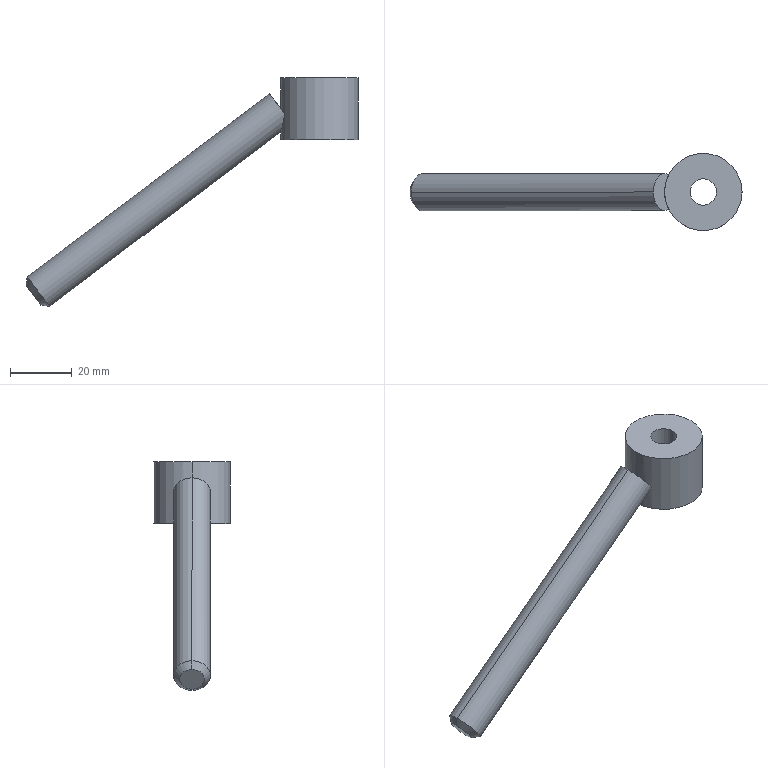Part | SolidWorks | features Chamfer 1, Extrusion 1, HoleWzd 1, Revolution 1 | 1 solid | 12 faces | box 107.206 x 25 x 73.855 mm | volume 19838 mm3 | cylinder 6 | plane 4 | cone 2 | commonest cylinder face diameters 8.5 x2 12 x2 25 x2
STEP:
#1=CARTESIAN_POINT('',(-94.706,0.,-57.081));
#2=VERTEX_POINT('',#1);
#3=CARTESIAN_POINT('',(-89.884,0.,-63.464));
#4=VERTEX_POINT('',#3);
#5=CARTESIAN_POINT('',(-92.295,0.,-60.273));
#6=DIRECTION('',(-0.7979,0.,-0.6027));
#7=DIRECTION('',(-0.6027,0.,0.7979));
#8=AXIS2_PLACEMENT_3D('',#5,#6,#7);
#9=CIRCLE('',#8,4.);
#10=EDGE_CURVE('',#2,#4,#9,.T.);
#11=ORIENTED_EDGE('',*,*,#10,.F.);
#12=CARTESIAN_POINT('',(-94.315,0.,-54.28));
#13=VERTEX_POINT('',#12);
#14=CARTESIAN_POINT('',(-94.315,0.,-54.28));
#15=DIRECTION('',(0.138,0.,0.9904));
#16=VECTOR('',#15,1000.);
#17=LINE('',#14,#16);
#18=EDGE_CURVE('',#2,#13,#17,.T.);
#19=ORIENTED_EDGE('',*,*,#18,.T.);
#20=CARTESIAN_POINT('',(-87.082,0.,-63.855));
#21=VERTEX_POINT('',#20);
#22=CARTESIAN_POINT('',(-90.699,0.,-59.067));
#23=DIRECTION('',(0.7979,0.,0.6027));
#24=DIRECTION('',(-0.6027,0.,0.7979));
#25=AXIS2_PLACEMENT_3D('',#22,#23,#24);
#26=CIRCLE('',#25,6.);
#27=EDGE_CURVE('',#21,#13,#26,.T.);
#28=ORIENTED_EDGE('',*,*,#27,.F.);
#29=CARTESIAN_POINT('',(-87.082,0.,-63.855));
#30=DIRECTION('',(0.9904,0.,-0.138));
#31=VECTOR('',#30,1000.);
#32=LINE('',#29,#31);
#33=EDGE_CURVE('',#4,#21,#32,.T.);
#34=ORIENTED_EDGE('',*,*,#33,.F.);
#35=EDGE_LOOP('',(#11,#19,#28,#34));
#36=FACE_OUTER_BOUND('',#35,.T.);
#37=CARTESIAN_POINT('',(-90.699,0.,-59.067));
#38=DIRECTION('',(0.7979,0.,0.6027));
#39=DIRECTION('',(0.6027,0.,-0.7979));
#40=AXIS2_PLACEMENT_3D('',#37,#38,#39);
#41=CONICAL_SURFACE('',#40,6.,0.7854);
#42=ADVANCED_FACE('',(#36),#41,.T.);
#43=ORIENTED_EDGE('',*,*,#27,.T.);
#44=CARTESIAN_POINT('',(-16.116,0.,4.788));
#45=VERTEX_POINT('',#44);
#46=CARTESIAN_POINT('',(-16.116,0.,4.788));
#47=DIRECTION('',(0.7979,0.,0.6027));
#48=VECTOR('',#47,1000.);
#49=LINE('',#46,#48);
#50=EDGE_CURVE('',#13,#45,#49,.T.);
#51=ORIENTED_EDGE('',*,*,#50,.T.);
#52=CARTESIAN_POINT('',(-11.182,5.587,-1.745));
#53=VERTEX_POINT('',#52);
#54=CARTESIAN_POINT('',(-12.5,0.,0.));
#55=DIRECTION('',(0.7979,0.,0.6027));
#56=DIRECTION('',(0.6027,0.,-0.7979));
#57=AXIS2_PLACEMENT_3D('',#54,#55,#56);
#58=CIRCLE('',#57,6.);
#59=EDGE_CURVE('',#53,#45,#58,.T.);
#60=ORIENTED_EDGE('',*,*,#59,.F.);
#61=CARTESIAN_POINT('',(-12.5,0.,-7.519));
#62=VERTEX_POINT('',#61);
#63=CARTESIAN_POINT('',(-12.5,0.,-7.519));
#64=CARTESIAN_POINT('',(-12.5,0.1816,-7.519));
#65=CARTESIAN_POINT('',(-12.496,0.362,-7.506));
#66=CARTESIAN_POINT('',(-12.481,0.7202,-7.454));
#67=CARTESIAN_POINT('',(-12.469,0.8992,-7.414));
#68=CARTESIAN_POINT('',(-12.424,1.424,-7.26));
#69=CARTESIAN_POINT('',(-12.38,1.753,-7.113));
#70=CARTESIAN_POINT('',(-12.276,2.379,-6.746));
#71=CARTESIAN_POINT('',(-12.215,2.666,-6.532));
#72=CARTESIAN_POINT('',(-12.087,3.199,-6.061));
#73=CARTESIAN_POINT('',(-12.018,3.446,-5.802));
#74=CARTESIAN_POINT('',(-11.807,4.131,-4.978));
#75=CARTESIAN_POINT('',(-11.665,4.505,-4.379));
#76=CARTESIAN_POINT('',(-11.466,4.98,-3.426));
#77=CARTESIAN_POINT('',(-11.402,5.124,-3.096));
#78=CARTESIAN_POINT('',(-11.284,5.38,-2.428));
#79=CARTESIAN_POINT('',(-11.23,5.491,-2.089));
#80=CARTESIAN_POINT('',(-11.182,5.587,-1.745));
#81=B_SPLINE_CURVE_WITH_KNOTS('',3,(#63,#64,#65,#66,#67,#68,#69,#70,#71,#72,#73,#74,#75,#76,#77,#78,#79,#80),.UNSPECIFIED.,.F.,.F.,(4,2,2,2,2,2,2,2,4),(0.02154,0.02208,0.02263,0.02371,0.02479,0.02588,0.02804,0.02913,0.03021),.UNSPECIFIED.);
#82=EDGE_CURVE('',#62,#53,#81,.T.);
#83=ORIENTED_EDGE('',*,*,#82,.F.);
#84=CARTESIAN_POINT('',(-8.884,0.,-4.788));
#85=DIRECTION('',(0.7979,0.,0.6027));
#86=VECTOR('',#85,1000.);
#87=LINE('',#84,#86);
#88=EDGE_CURVE('',#21,#62,#87,.T.);
#89=ORIENTED_EDGE('',*,*,#88,.F.);
#90=EDGE_LOOP('',(#43,#51,#60,#83,#89));
#91=FACE_OUTER_BOUND('',#90,.T.);
#92=CARTESIAN_POINT('',(-12.5,0.,0.));
#93=DIRECTION('',(0.7979,0.,0.6027));
#94=DIRECTION('',(0.6027,0.,-0.7979));
#95=AXIS2_PLACEMENT_3D('',#92,#93,#94);
#96=CYLINDRICAL_SURFACE('',#95,6.);
#97=ADVANCED_FACE('',(#91),#96,.T.);
#98=CARTESIAN_POINT('',(-4.25,0.,-10.));
#99=VERTEX_POINT('',#98);
#100=CARTESIAN_POINT('',(4.25,0.,-10.));
#101=VERTEX_POINT('',#100);
#102=CARTESIAN_POINT('',(0.,0.,-10.));
#103=DIRECTION('',(0.,0.,1.));
#104=DIRECTION('',(1.,0.,0.));
#105=AXIS2_PLACEMENT_3D('',#102,#103,#104);
#106=CIRCLE('',#105,4.25);
#107=EDGE_CURVE('',#99,#101,#106,.T.);
#108=ORIENTED_EDGE('',*,*,#107,.F.);
#109=CARTESIAN_POINT('',(-4.25,0.,10.));
#110=VERTEX_POINT('',#109);
#111=CARTESIAN_POINT('',(-4.25,0.,10.));
#112=DIRECTION('',(0.,0.,1.));
#113=VECTOR('',#112,1000.);
#114=LINE('',#111,#113);
#115=EDGE_CURVE('',#99,#110,#114,.T.);
#116=ORIENTED_EDGE('',*,*,#115,.T.);
#117=CARTESIAN_POINT('',(4.25,0.,10.));
#118=VERTEX_POINT('',#117);
#119=CARTESIAN_POINT('',(0.,0.,10.));
#120=DIRECTION('',(0.,0.,1.));
#121=DIRECTION('',(1.,0.,0.));
#122=AXIS2_PLACEMENT_3D('',#119,#120,#121);
#123=CIRCLE('',#122,4.25);
#124=EDGE_CURVE('',#110,#118,#123,.T.);
#125=ORIENTED_EDGE('',*,*,#124,.T.);
#126=CARTESIAN_POINT('',(4.25,0.,10.));
#127=DIRECTION('',(0.,0.,1.));
#128=VECTOR('',#127,1000.);
#129=LINE('',#126,#128);
#130=EDGE_CURVE('',#101,#118,#129,.T.);
#131=ORIENTED_EDGE('',*,*,#130,.F.);
#132=EDGE_LOOP('',(#108,#116,#125,#131));
#133=FACE_OUTER_BOUND('',#132,.T.);
#134=CARTESIAN_POINT('',(0.,0.,10.));
#135=DIRECTION('',(0.,0.,1.));
#136=DIRECTION('',(1.,0.,0.));
#137=AXIS2_PLACEMENT_3D('',#134,#135,#136);
#138=CYLINDRICAL_SURFACE('',#137,4.25);
#139=ADVANCED_FACE('',(#133),#138,.F.);
#140=CARTESIAN_POINT('',(12.5,0.,10.));
#141=VERTEX_POINT('',#140);
#142=CARTESIAN_POINT('',(-12.5,0.,10.));
#143=VERTEX_POINT('',#142);
#144=CARTESIAN_POINT('',(0.,0.,10.));
#145=DIRECTION('',(0.,0.,1.));
#146=DIRECTION('',(1.,0.,0.));
#147=AXIS2_PLACEMENT_3D('',#144,#145,#146);
#148=CIRCLE('',#147,12.5);
#149=EDGE_CURVE('',#141,#143,#148,.T.);
#150=ORIENTED_EDGE('',*,*,#149,.F.);
#151=CARTESIAN_POINT('',(12.5,0.,-10.));
#152=VERTEX_POINT('',#151);
#153=CARTESIAN_POINT('',(12.5,0.,10.));
#154=DIRECTION('',(0.,0.,-1.));
#155=VECTOR('',#154,1000.);
#156=LINE('',#153,#155);
#157=EDGE_CURVE('',#141,#152,#156,.T.);
#158=ORIENTED_EDGE('',*,*,#157,.T.);
#159=CARTESIAN_POINT('',(-12.5,0.,-10.));
#160=VERTEX_POINT('',#159);
#161=CARTESIAN_POINT('',(0.,0.,-10.));
#162=DIRECTION('',(0.,0.,1.));
#163=DIRECTION('',(1.,0.,0.));
#164=AXIS2_PLACEMENT_3D('',#161,#162,#163);
#165=CIRCLE('',#164,12.5);
#166=EDGE_CURVE('',#152,#160,#165,.T.);
#167=ORIENTED_EDGE('',*,*,#166,.T.);
#168=CARTESIAN_POINT('',(-12.5,0.,10.));
#169=DIRECTION('',(0.,0.,-1.));
#170=VECTOR('',#169,1000.);
#171=LINE('',#168,#170);
#172=EDGE_CURVE('',#62,#160,#171,.T.);
#173=ORIENTED_EDGE('',*,*,#172,.F.);
#174=ORIENTED_EDGE('',*,*,#82,.T.);
#175=CARTESIAN_POINT('',(-12.5,0.,0.));
#176=VERTEX_POINT('',#175);
#177=CARTESIAN_POINT('',(-11.182,5.587,-1.745));
#178=CARTESIAN_POINT('',(-12.053,3.844,-0.5923));
#179=CARTESIAN_POINT('',(-12.5,1.948,0.));
#180=CARTESIAN_POINT('',(-12.5,0.,0.));
#181=(BOUNDED_CURVE()B_SPLINE_CURVE(3,(#177,#178,#179,#180),.UNSPECIFIED.,.F.,.F.)B_SPLINE_CURVE_WITH_KNOTS((4,4),(2.678,3.142),.UNSPECIFIED.)CURVE()GEOMETRIC_REPRESENTATION_ITEM()RATIONAL_B_SPLINE_CURVE((1.,0.9822,0.9822,1.))REPRESENTATION_ITEM(''));
#182=EDGE_CURVE('',#53,#176,#181,.T.);
#183=ORIENTED_EDGE('',*,*,#182,.T.);
#184=CARTESIAN_POINT('',(-12.5,0.,10.));
#185=DIRECTION('',(0.,0.,-1.));
#186=VECTOR('',#185,1000.);
#187=LINE('',#184,#186);
#188=EDGE_CURVE('',#143,#176,#187,.T.);
#189=ORIENTED_EDGE('',*,*,#188,.F.);
#190=EDGE_LOOP('',(#150,#158,#167,#173,#174,#183,#189));
#191=FACE_OUTER_BOUND('',#190,.T.);
#192=CARTESIAN_POINT('',(0.,0.,10.));
#193=DIRECTION('',(0.,0.,-1.));
#194=DIRECTION('',(-1.,0.,0.));
#195=AXIS2_PLACEMENT_3D('',#192,#193,#194);
#196=CYLINDRICAL_SURFACE('',#195,12.5);
#197=ADVANCED_FACE('',(#191),#196,.T.);
#198=ORIENTED_EDGE('',*,*,#157,.F.);
#199=CARTESIAN_POINT('',(0.,0.,10.));
#200=DIRECTION('',(0.,0.,1.));
#201=DIRECTION('',(1.,0.,0.));
#202=AXIS2_PLACEMENT_3D('',#199,#200,#201);
#203=CIRCLE('',#202,12.5);
#204=EDGE_CURVE('',#143,#141,#203,.T.);
#205=ORIENTED_EDGE('',*,*,#204,.F.);
#206=ORIENTED_EDGE('',*,*,#188,.T.);
#207=CARTESIAN_POINT('',(-11.182,-5.587,-1.745));
#208=VERTEX_POINT('',#207);
#209=CARTESIAN_POINT('',(-12.5,0.,0.));
#210=CARTESIAN_POINT('',(-12.5,-1.948,0.));
#211=CARTESIAN_POINT('',(-12.053,-3.844,-0.5923));
#212=CARTESIAN_POINT('',(-11.182,-5.587,-1.745));
#213=(BOUNDED_CURVE()B_SPLINE_CURVE(3,(#209,#210,#211,#212),.UNSPECIFIED.,.F.,.F.)B_SPLINE_CURVE_WITH_KNOTS((4,4),(3.142,3.605),.UNSPECIFIED.)CURVE()GEOMETRIC_REPRESENTATION_ITEM()RATIONAL_B_SPLINE_CURVE((1.,0.9822,0.9822,1.))REPRESENTATION_ITEM(''));
#214=EDGE_CURVE('',#176,#208,#213,.T.);
#215=ORIENTED_EDGE('',*,*,#214,.T.);
#216=CARTESIAN_POINT('',(-11.182,-5.587,-1.745));
#217=CARTESIAN_POINT('',(-11.279,-5.393,-2.439));
#218=CARTESIAN_POINT('',(-11.4,-5.14,-3.105));
#219=CARTESIAN_POINT('',(-11.664,-4.508,-4.374));
#220=CARTESIAN_POINT('',(-11.809,-4.126,-4.985));
#221=CARTESIAN_POINT('',(-12.018,-3.446,-5.802));
#222=CARTESIAN_POINT('',(-12.087,-3.2,-6.06));
#223=CARTESIAN_POINT('',(-12.216,-2.662,-6.535));
#224=CARTESIAN_POINT('',(-12.276,-2.374,-6.749));
#225=CARTESIAN_POINT('',(-12.38,-1.757,-7.111));
#226=CARTESIAN_POINT('',(-12.424,-1.421,-7.261));
#227=CARTESIAN_POINT('',(-12.469,-0.9017,-7.413));
#228=CARTESIAN_POINT('',(-12.48,-0.7253,-7.453));
#229=CARTESIAN_POINT('',(-12.496,-0.3657,-7.506));
#230=CARTESIAN_POINT('',(-12.5,-0.1815,-7.519));
#231=CARTESIAN_POINT('',(-12.5,0.,-7.519));
#232=B_SPLINE_CURVE_WITH_KNOTS('',3,(#216,#217,#218,#219,#220,#221,#222,#223,#224,#225,#226,#227,#228,#229,#230,#231),.UNSPECIFIED.,.F.,.F.,(4,2,2,2,2,2,2,4),(0.01289,0.01505,0.01721,0.0183,0.01938,0.02046,0.021,0.02154),.UNSPECIFIED.);
#233=EDGE_CURVE('',#208,#62,#232,.T.);
#234=ORIENTED_EDGE('',*,*,#233,.T.);
#235=ORIENTED_EDGE('',*,*,#172,.T.);
#236=CARTESIAN_POINT('',(0.,0.,-10.));
#237=DIRECTION('',(0.,0.,1.));
#238=DIRECTION('',(1.,0.,0.));
#239=AXIS2_PLACEMENT_3D('',#236,#237,#238);
#240=CIRCLE('',#239,12.5);
#241=EDGE_CURVE('',#160,#152,#240,.T.);
#242=ORIENTED_EDGE('',*,*,#241,.T.);
#243=EDGE_LOOP('',(#198,#205,#206,#215,#234,#235,#242));
#244=FACE_OUTER_BOUND('',#243,.T.);
#245=CARTESIAN_POINT('',(0.,0.,10.));
#246=DIRECTION('',(0.,0.,-1.));
#247=DIRECTION('',(-1.,0.,0.));
#248=AXIS2_PLACEMENT_3D('',#245,#246,#247);
#249=CYLINDRICAL_SURFACE('',#248,12.5);
#250=ADVANCED_FACE('',(#244),#249,.T.);
#251=CARTESIAN_POINT('',(0.,0.,10.));
#252=DIRECTION('',(0.,0.,1.));
#253=DIRECTION('',(1.,0.,0.));
#254=AXIS2_PLACEMENT_3D('',#251,#252,#253);
#255=CIRCLE('',#254,4.25);
#256=EDGE_CURVE('',#118,#110,#255,.T.);
#257=ORIENTED_EDGE('',*,*,#256,.F.);
#258=ORIENTED_EDGE('',*,*,#124,.F.);
#259=EDGE_LOOP('',(#257,#258));
#260=FACE_BOUND('',#259,.T.);
#261=ORIENTED_EDGE('',*,*,#204,.T.);
#262=ORIENTED_EDGE('',*,*,#149,.T.);
#263=EDGE_LOOP('',(#261,#262));
#264=FACE_OUTER_BOUND('',#263,.T.);
#265=CARTESIAN_POINT('',(0.,0.,10.));
#266=DIRECTION('',(0.,0.,1.));
#267=DIRECTION('',(1.,0.,0.));
#268=AXIS2_PLACEMENT_3D('',#265,#266,#267);
#269=PLANE('',#268);
#270=ADVANCED_FACE('',(#260,#264),#269,.T.);
#271=CARTESIAN_POINT('',(0.,0.,-10.));
#272=DIRECTION('',(0.,0.,1.));
#273=DIRECTION('',(1.,0.,0.));
#274=AXIS2_PLACEMENT_3D('',#271,#272,#273);
#275=CIRCLE('',#274,4.25);
#276=EDGE_CURVE('',#101,#99,#275,.T.);
#277=ORIENTED_EDGE('',*,*,#276,.T.);
#278=ORIENTED_EDGE('',*,*,#107,.T.);
#279=EDGE_LOOP('',(#277,#278));
#280=FACE_BOUND('',#279,.T.);
#281=ORIENTED_EDGE('',*,*,#241,.F.);
#282=ORIENTED_EDGE('',*,*,#166,.F.);
#283=EDGE_LOOP('',(#281,#282));
#284=FACE_OUTER_BOUND('',#283,.T.);
#285=CARTESIAN_POINT('',(0.,0.,-10.));
#286=DIRECTION('',(0.,0.,1.));
#287=DIRECTION('',(1.,0.,0.));
#288=AXIS2_PLACEMENT_3D('',#285,#286,#287);
#289=PLANE('',#288);
#290=ADVANCED_FACE('',(#280,#284),#289,.F.);
#291=ORIENTED_EDGE('',*,*,#115,.F.);
#292=ORIENTED_EDGE('',*,*,#276,.F.);
#293=ORIENTED_EDGE('',*,*,#130,.T.);
#294=ORIENTED_EDGE('',*,*,#256,.T.);
#295=EDGE_LOOP('',(#291,#292,#293,#294));
#296=FACE_OUTER_BOUND('',#295,.T.);
#297=CARTESIAN_POINT('',(0.,0.,10.));
#298=DIRECTION('',(0.,0.,1.));
#299=DIRECTION('',(1.,0.,0.));
#300=AXIS2_PLACEMENT_3D('',#297,#298,#299);
#301=CYLINDRICAL_SURFACE('',#300,4.25);
#302=ADVANCED_FACE('',(#296),#301,.F.);
#303=ORIENTED_EDGE('',*,*,#50,.F.);
#304=CARTESIAN_POINT('',(-90.699,0.,-59.067));
#305=DIRECTION('',(0.7979,0.,0.6027));
#306=DIRECTION('',(-0.6027,0.,0.7979));
#307=AXIS2_PLACEMENT_3D('',#304,#305,#306);
#308=CIRCLE('',#307,6.);
#309=EDGE_CURVE('',#13,#21,#308,.T.);
#310=ORIENTED_EDGE('',*,*,#309,.T.);
#311=ORIENTED_EDGE('',*,*,#88,.T.);
#312=ORIENTED_EDGE('',*,*,#233,.F.);
#313=CARTESIAN_POINT('',(-12.5,0.,0.));
#314=DIRECTION('',(0.7979,0.,0.6027));
#315=DIRECTION('',(0.6027,0.,-0.7979));
#316=AXIS2_PLACEMENT_3D('',#313,#314,#315);
#317=CIRCLE('',#316,6.);
#318=EDGE_CURVE('',#45,#208,#317,.T.);
#319=ORIENTED_EDGE('',*,*,#318,.F.);
#320=EDGE_LOOP('',(#303,#310,#311,#312,#319));
#321=FACE_OUTER_BOUND('',#320,.T.);
#322=CARTESIAN_POINT('',(-12.5,0.,0.));
#323=DIRECTION('',(0.7979,0.,0.6027));
#324=DIRECTION('',(0.6027,0.,-0.7979));
#325=AXIS2_PLACEMENT_3D('',#322,#323,#324);
#326=CYLINDRICAL_SURFACE('',#325,6.);
#327=ADVANCED_FACE('',(#321),#326,.T.);
#328=ORIENTED_EDGE('',*,*,#182,.F.);
#329=ORIENTED_EDGE('',*,*,#59,.T.);
#330=ORIENTED_EDGE('',*,*,#318,.T.);
#331=ORIENTED_EDGE('',*,*,#214,.F.);
#332=EDGE_LOOP('',(#328,#329,#330,#331));
#333=FACE_OUTER_BOUND('',#332,.T.);
#334=CARTESIAN_POINT('',(-12.5,0.,0.));
#335=DIRECTION('',(0.7979,0.,0.6027));
#336=DIRECTION('',(0.6027,0.,-0.7979));
#337=AXIS2_PLACEMENT_3D('',#334,#335,#336);
#338=PLANE('',#337);
#339=ADVANCED_FACE('',(#333),#338,.T.);
#340=CARTESIAN_POINT('',(-92.295,0.,-60.273));
#341=DIRECTION('',(-0.7979,0.,-0.6027));
#342=DIRECTION('',(-0.6027,0.,0.7979));
#343=AXIS2_PLACEMENT_3D('',#340,#341,#342);
#344=CIRCLE('',#343,4.);
#345=EDGE_CURVE('',#4,#2,#344,.T.);
#346=ORIENTED_EDGE('',*,*,#345,.T.);
#347=ORIENTED_EDGE('',*,*,#10,.T.);
#348=EDGE_LOOP('',(#346,#347));
#349=FACE_OUTER_BOUND('',#348,.T.);
#350=CARTESIAN_POINT('',(-92.295,0.,-60.273));
#351=DIRECTION('',(-0.7979,0.,-0.6027));
#352=DIRECTION('',(-0.6027,0.,0.7979));
#353=AXIS2_PLACEMENT_3D('',#350,#351,#352);
#354=PLANE('',#353);
#355=ADVANCED_FACE('',(#349),#354,.T.);
#356=ORIENTED_EDGE('',*,*,#18,.F.);
#357=ORIENTED_EDGE('',*,*,#345,.F.);
#358=ORIENTED_EDGE('',*,*,#33,.T.);
#359=ORIENTED_EDGE('',*,*,#309,.F.);
#360=EDGE_LOOP('',(#356,#357,#358,#359));
#361=FACE_OUTER_BOUND('',#360,.T.);
#362=CARTESIAN_POINT('',(-90.699,0.,-59.067));
#363=DIRECTION('',(0.7979,0.,0.6027));
#364=DIRECTION('',(0.6027,0.,-0.7979));
#365=AXIS2_PLACEMENT_3D('',#362,#363,#364);
#366=CONICAL_SURFACE('',#365,6.,0.7854);
#367=ADVANCED_FACE('',(#361),#366,.T.);
#368=CLOSED_SHELL('',(#42,#97,#139,#197,#250,#270,#290,#302,#327,#339,#355,#367));
#369=MANIFOLD_SOLID_BREP('',#368);
#370=CARTESIAN_POINT('',(0.,0.,0.));
#371=DIRECTION('',(0.,0.,1.));
#372=DIRECTION('',(1.,0.,0.));
#373=AXIS2_PLACEMENT_3D('',#370,#371,#372);
#374=(LENGTH_UNIT()NAMED_UNIT(*)SI_UNIT(.MILLI.,.METRE.));
#375=UNCERTAINTY_MEASURE_WITH_UNIT(LENGTH_MEASURE(0.00001),#374,'','');
#376=(NAMED_UNIT(*)PLANE_ANGLE_UNIT()SI_UNIT($,.RADIAN.));
#377=(NAMED_UNIT(*)SI_UNIT($,.STERADIAN.)SOLID_ANGLE_UNIT());
#378=(GEOMETRIC_REPRESENTATION_CONTEXT(3)GLOBAL_UNCERTAINTY_ASSIGNED_CONTEXT((#375))GLOBAL_UNIT_ASSIGNED_CONTEXT((#374,#376,#377))REPRESENTATION_CONTEXT('',''));
#379=ADVANCED_BREP_SHAPE_REPRESENTATION('',(#369,#373),#378);